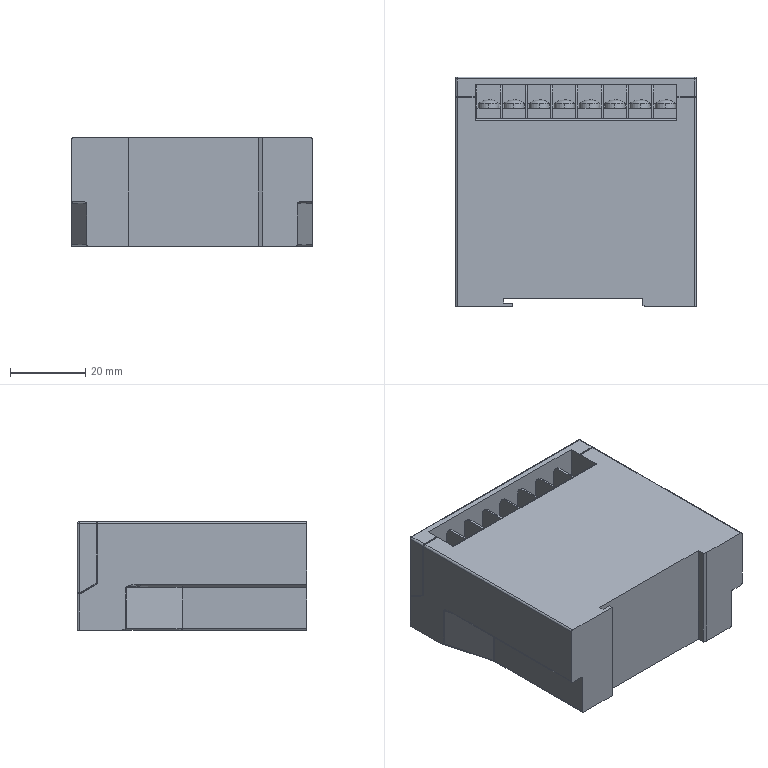Part | STEP file | SS5V1-16S3AD-08B-N1_EX120 SI Unit | 1 solid | 219 faces | box 64 x 61 x 28.8 mm | volume 102624 mm3 | plane 115 | cylinder 64 | cone 24 | sphere 12 | spline 2 | torus 2 | commonest cylinder face diameters 1 x24 5.5 x16 4 x8 0.25 x4 0.75 x4 1.75 x4